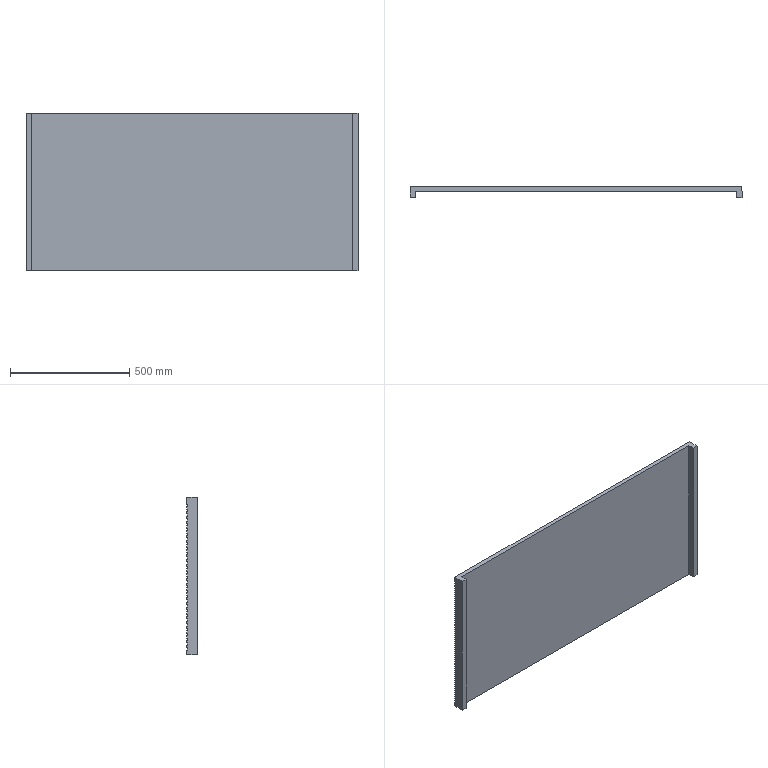Part | SolidWorks | features Extrusion 1, ICE 1, LPattern 1 | 1 solid | 134 faces | box 1390 x 45 x 660 mm | volume 17341000 mm3 | plane 134